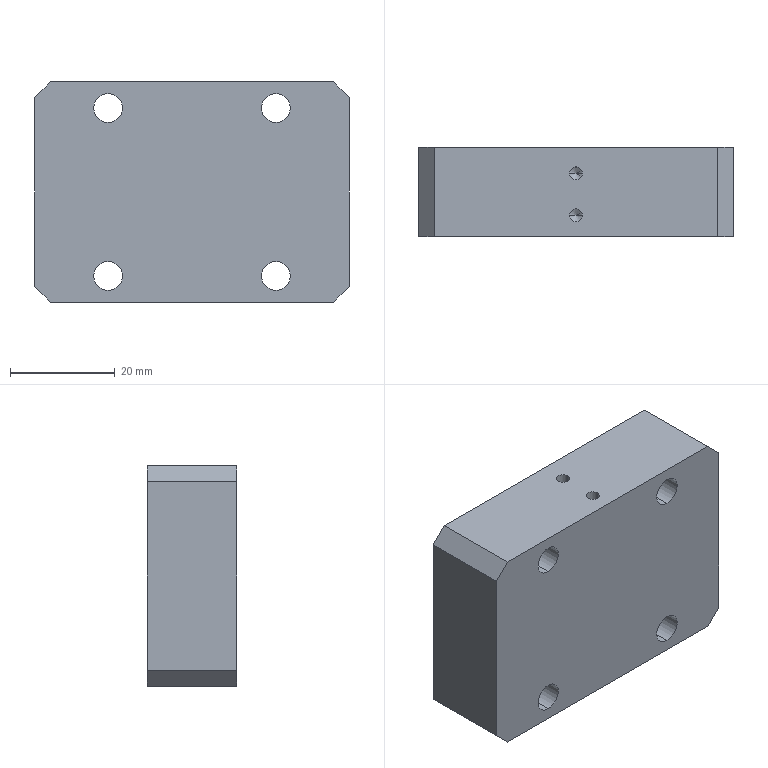Part | STEP file | 0-19 Pad block | 1 solid | 26 faces | box 60 x 17 x 42 mm | volume 40842 mm3 | cylinder 12 | plane 10 | cone 4 | commonest cylinder face diameters 5.5 x8 2.5 x4